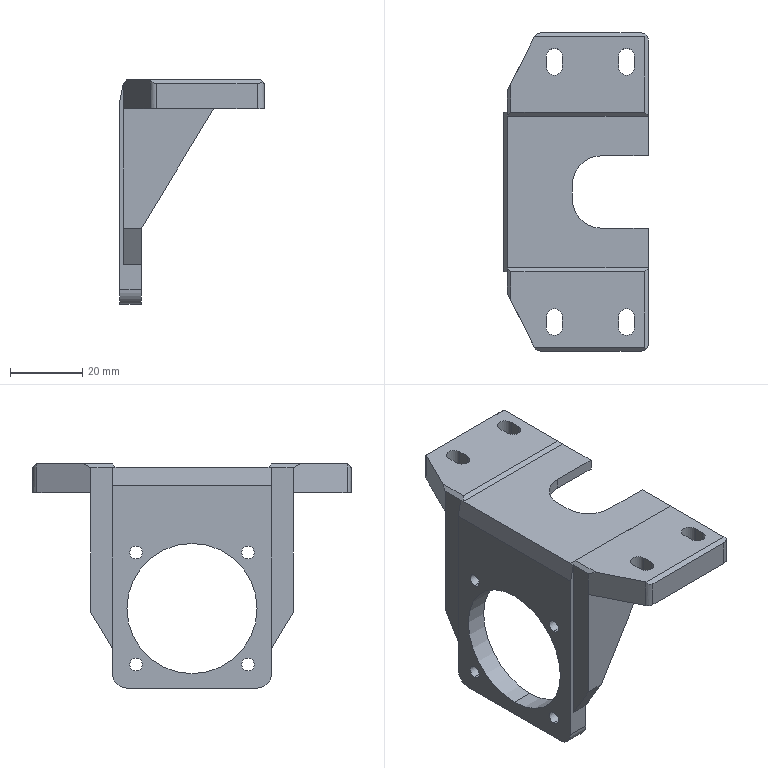Part | SolidWorks | features ICE 9, Chamfer 4, Fillet 3, Extrusion 1, HoleWzd 1 | 1 solid | 74 faces | box 40 x 88 x 62 mm | volume 31074 mm3 | plane 47 | cylinder 27 | commonest cylinder face diameters 3.5 x8 4.4 x8 4 x4 8 x3 16 x2 36 x2